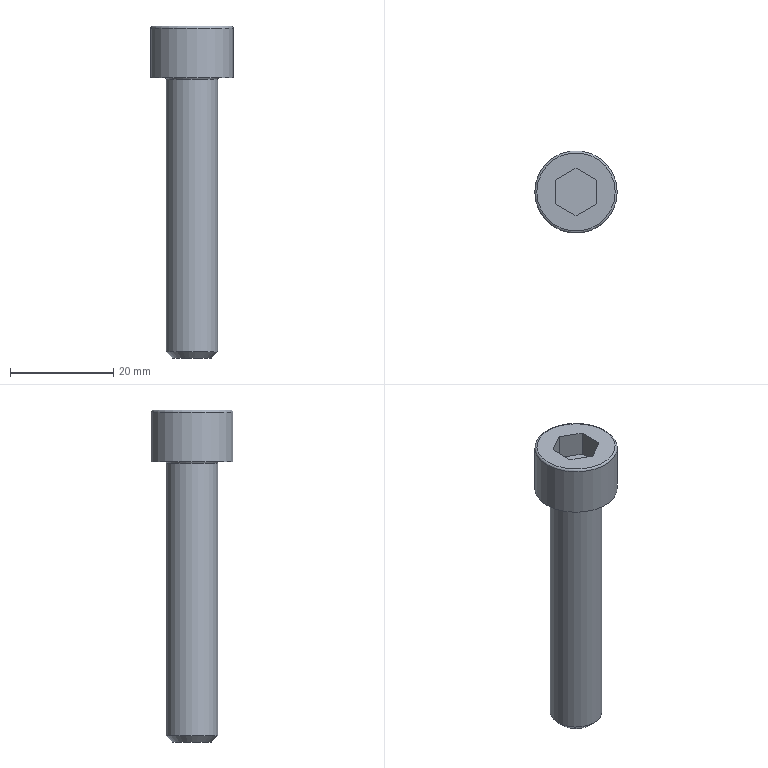Part | STEP file | solid 156 | 1 solid | 15 faces | box 16 x 16 x 64.4 mm | volume 5983 mm3 | plane 10 | cylinder 2 | torus 2 | cone 1 | commonest cylinder face diameters 10 x1 16 x1